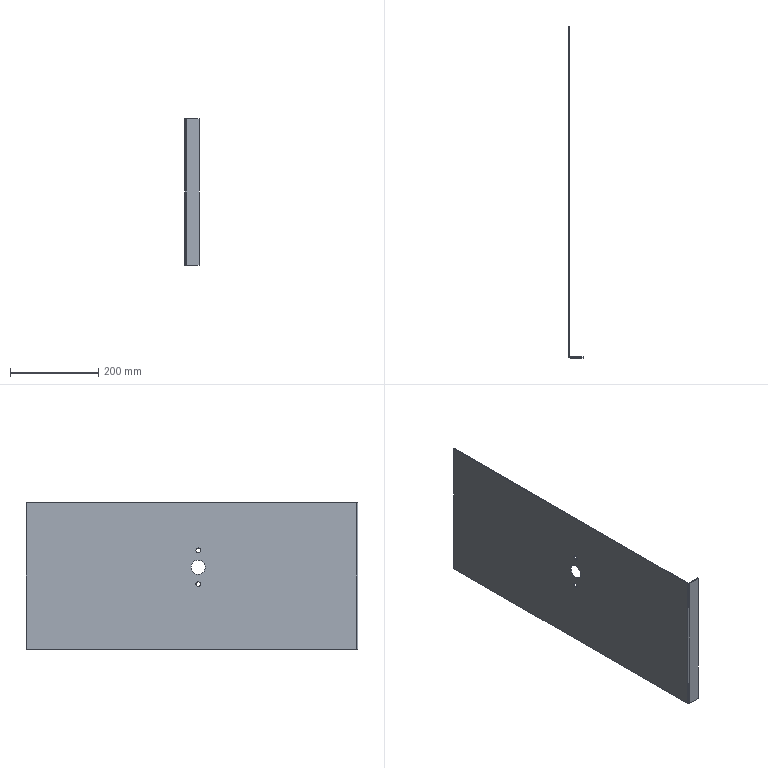Part | SolidWorks | features FlatPattern 1, ICE 1, SMBaseFlange 1, SheetMetal 1 | 1 solid | 20 faces | box 32 x 752 x 333 mm | volume 518361 mm3 | plane 12 | cylinder 8 | commonest cylinder face diameters 10.5 x4 32 x2 1.473 x1 5.473 x1
STEP:
#1=CARTESIAN_POINT('',(0.,87.126,63.5));
#2=VERTEX_POINT('',#1);
#3=CARTESIAN_POINT('',(0.,87.126,53.));
#4=VERTEX_POINT('',#3);
#5=CARTESIAN_POINT('',(0.,87.126,58.25));
#6=DIRECTION('',(1.,0.,0.));
#7=DIRECTION('',(0.,0.,-1.));
#8=AXIS2_PLACEMENT_3D('',#5,#6,#7);
#9=CIRCLE('',#8,5.25);
#10=EDGE_CURVE('',#2,#4,#9,.T.);
#11=ORIENTED_EDGE('',*,*,#10,.T.);
#12=CARTESIAN_POINT('',(-2.,87.126,53.));
#13=VERTEX_POINT('',#12);
#14=CARTESIAN_POINT('',(8.,87.126,53.));
#15=DIRECTION('',(-1.,0.,0.));
#16=VECTOR('',#15,1000.);
#17=LINE('',#14,#16);
#18=EDGE_CURVE('',#4,#13,#17,.T.);
#19=ORIENTED_EDGE('',*,*,#18,.T.);
#20=CARTESIAN_POINT('',(-2.,87.126,63.5));
#21=VERTEX_POINT('',#20);
#22=CARTESIAN_POINT('',(-2.,87.126,58.25));
#23=DIRECTION('',(-1.,0.,0.));
#24=DIRECTION('',(0.,0.,1.));
#25=AXIS2_PLACEMENT_3D('',#22,#23,#24);
#26=CIRCLE('',#25,5.25);
#27=EDGE_CURVE('',#13,#21,#26,.T.);
#28=ORIENTED_EDGE('',*,*,#27,.T.);
#29=CARTESIAN_POINT('',(8.,87.126,63.5));
#30=DIRECTION('',(-1.,0.,0.));
#31=VECTOR('',#30,1000.);
#32=LINE('',#29,#31);
#33=EDGE_CURVE('',#2,#21,#32,.T.);
#34=ORIENTED_EDGE('',*,*,#33,.F.);
#35=EDGE_LOOP('',(#11,#19,#28,#34));
#36=FACE_OUTER_BOUND('',#35,.T.);
#37=CARTESIAN_POINT('',(8.,87.126,58.25));
#38=DIRECTION('',(-1.,0.,0.));
#39=DIRECTION('',(0.,0.,1.));
#40=AXIS2_PLACEMENT_3D('',#37,#38,#39);
#41=CYLINDRICAL_SURFACE('',#40,5.25);
#42=ADVANCED_FACE('',(#36),#41,.F.);
#43=CARTESIAN_POINT('',(0.,87.126,-13.));
#44=VERTEX_POINT('',#43);
#45=CARTESIAN_POINT('',(0.,87.126,-23.5));
#46=VERTEX_POINT('',#45);
#47=CARTESIAN_POINT('',(0.,87.126,-18.25));
#48=DIRECTION('',(1.,0.,0.));
#49=DIRECTION('',(0.,0.,-1.));
#50=AXIS2_PLACEMENT_3D('',#47,#48,#49);
#51=CIRCLE('',#50,5.25);
#52=EDGE_CURVE('',#44,#46,#51,.T.);
#53=ORIENTED_EDGE('',*,*,#52,.T.);
#54=CARTESIAN_POINT('',(-2.,87.126,-23.5));
#55=VERTEX_POINT('',#54);
#56=CARTESIAN_POINT('',(8.,87.126,-23.5));
#57=DIRECTION('',(-1.,0.,0.));
#58=VECTOR('',#57,1000.);
#59=LINE('',#56,#58);
#60=EDGE_CURVE('',#46,#55,#59,.T.);
#61=ORIENTED_EDGE('',*,*,#60,.T.);
#62=CARTESIAN_POINT('',(-2.,87.126,-13.));
#63=VERTEX_POINT('',#62);
#64=CARTESIAN_POINT('',(-2.,87.126,-18.25));
#65=DIRECTION('',(-1.,0.,0.));
#66=DIRECTION('',(0.,0.,1.));
#67=AXIS2_PLACEMENT_3D('',#64,#65,#66);
#68=CIRCLE('',#67,5.25);
#69=EDGE_CURVE('',#55,#63,#68,.T.);
#70=ORIENTED_EDGE('',*,*,#69,.T.);
#71=CARTESIAN_POINT('',(8.,87.126,-13.));
#72=DIRECTION('',(-1.,0.,0.));
#73=VECTOR('',#72,1000.);
#74=LINE('',#71,#73);
#75=EDGE_CURVE('',#44,#63,#74,.T.);
#76=ORIENTED_EDGE('',*,*,#75,.F.);
#77=EDGE_LOOP('',(#53,#61,#70,#76));
#78=FACE_OUTER_BOUND('',#77,.T.);
#79=CARTESIAN_POINT('',(8.,87.126,-18.25));
#80=DIRECTION('',(-1.,0.,0.));
#81=DIRECTION('',(0.,0.,1.));
#82=AXIS2_PLACEMENT_3D('',#79,#80,#81);
#83=CYLINDRICAL_SURFACE('',#82,5.25);
#84=ADVANCED_FACE('',(#78),#83,.F.);
#85=CARTESIAN_POINT('',(0.,87.126,36.));
#86=VERTEX_POINT('',#85);
#87=CARTESIAN_POINT('',(0.,87.126,4.));
#88=VERTEX_POINT('',#87);
#89=CARTESIAN_POINT('',(0.,87.126,20.));
#90=DIRECTION('',(1.,0.,0.));
#91=DIRECTION('',(0.,0.,-1.));
#92=AXIS2_PLACEMENT_3D('',#89,#90,#91);
#93=CIRCLE('',#92,16.);
#94=EDGE_CURVE('',#86,#88,#93,.T.);
#95=ORIENTED_EDGE('',*,*,#94,.T.);
#96=CARTESIAN_POINT('',(-2.,87.126,4.));
#97=VERTEX_POINT('',#96);
#98=CARTESIAN_POINT('',(8.,87.126,4.));
#99=DIRECTION('',(-1.,0.,0.));
#100=VECTOR('',#99,1000.);
#101=LINE('',#98,#100);
#102=EDGE_CURVE('',#88,#97,#101,.T.);
#103=ORIENTED_EDGE('',*,*,#102,.T.);
#104=CARTESIAN_POINT('',(-2.,87.126,36.));
#105=VERTEX_POINT('',#104);
#106=CARTESIAN_POINT('',(-2.,87.126,20.));
#107=DIRECTION('',(-1.,0.,0.));
#108=DIRECTION('',(0.,0.,1.));
#109=AXIS2_PLACEMENT_3D('',#106,#107,#108);
#110=CIRCLE('',#109,16.);
#111=EDGE_CURVE('',#97,#105,#110,.T.);
#112=ORIENTED_EDGE('',*,*,#111,.T.);
#113=CARTESIAN_POINT('',(8.,87.126,36.));
#114=DIRECTION('',(-1.,0.,0.));
#115=VECTOR('',#114,1000.);
#116=LINE('',#113,#115);
#117=EDGE_CURVE('',#86,#105,#116,.T.);
#118=ORIENTED_EDGE('',*,*,#117,.F.);
#119=EDGE_LOOP('',(#95,#103,#112,#118));
#120=FACE_OUTER_BOUND('',#119,.T.);
#121=CARTESIAN_POINT('',(8.,87.126,20.));
#122=DIRECTION('',(-1.,0.,0.));
#123=DIRECTION('',(0.,0.,1.));
#124=AXIS2_PLACEMENT_3D('',#121,#122,#123);
#125=CYLINDRICAL_SURFACE('',#124,16.);
#126=ADVANCED_FACE('',(#120),#125,.F.);
#127=CARTESIAN_POINT('',(0.7366,-272.664,166.5));
#128=VERTEX_POINT('',#127);
#129=CARTESIAN_POINT('',(0.7366,-274.664,166.5));
#130=VERTEX_POINT('',#129);
#131=CARTESIAN_POINT('',(0.7366,-272.664,166.5));
#132=DIRECTION('',(0.,-1.,0.));
#133=VECTOR('',#132,1000.);
#134=LINE('',#131,#133);
#135=EDGE_CURVE('',#128,#130,#134,.T.);
#136=ORIENTED_EDGE('',*,*,#135,.F.);
#137=CARTESIAN_POINT('',(0.,-271.928,166.5));
#138=VERTEX_POINT('',#137);
#139=CARTESIAN_POINT('',(0.7366,-271.928,166.5));
#140=DIRECTION('',(0.,0.,1.));
#141=DIRECTION('',(-1.,0.,0.));
#142=AXIS2_PLACEMENT_3D('',#139,#140,#141);
#143=CIRCLE('',#142,0.7366);
#144=EDGE_CURVE('',#138,#128,#143,.T.);
#145=ORIENTED_EDGE('',*,*,#144,.F.);
#146=CARTESIAN_POINT('',(-2.,-271.928,166.5));
#147=VERTEX_POINT('',#146);
#148=CARTESIAN_POINT('',(-2.,-271.928,166.5));
#149=DIRECTION('',(1.,0.,0.));
#150=VECTOR('',#149,1000.);
#151=LINE('',#148,#150);
#152=EDGE_CURVE('',#147,#138,#151,.T.);
#153=ORIENTED_EDGE('',*,*,#152,.F.);
#154=CARTESIAN_POINT('',(0.7366,-271.928,166.5));
#155=DIRECTION('',(0.,0.,1.));
#156=DIRECTION('',(1.,0.,0.));
#157=AXIS2_PLACEMENT_3D('',#154,#155,#156);
#158=CIRCLE('',#157,2.737);
#159=EDGE_CURVE('',#147,#130,#158,.T.);
#160=ORIENTED_EDGE('',*,*,#159,.T.);
#161=EDGE_LOOP('',(#136,#145,#153,#160));
#162=FACE_OUTER_BOUND('',#161,.T.);
#163=CARTESIAN_POINT('',(0.7366,-272.664,166.5));
#164=DIRECTION('',(0.,0.,1.));
#165=DIRECTION('',(1.,0.,0.));
#166=AXIS2_PLACEMENT_3D('',#163,#164,#165);
#167=PLANE('',#166);
#168=ADVANCED_FACE('',(#162),#167,.T.);
#169=CARTESIAN_POINT('',(30.,-272.664,166.5));
#170=VERTEX_POINT('',#169);
#171=CARTESIAN_POINT('',(0.,-272.664,166.5));
#172=DIRECTION('',(1.,0.,0.));
#173=VECTOR('',#172,1000.);
#174=LINE('',#171,#173);
#175=EDGE_CURVE('',#128,#170,#174,.T.);
#176=ORIENTED_EDGE('',*,*,#175,.F.);
#177=ORIENTED_EDGE('',*,*,#135,.T.);
#178=CARTESIAN_POINT('',(30.,-274.664,166.5));
#179=VERTEX_POINT('',#178);
#180=CARTESIAN_POINT('',(0.,-274.664,166.5));
#181=DIRECTION('',(1.,0.,0.));
#182=VECTOR('',#181,1000.);
#183=LINE('',#180,#182);
#184=EDGE_CURVE('',#130,#179,#183,.T.);
#185=ORIENTED_EDGE('',*,*,#184,.T.);
#186=CARTESIAN_POINT('',(30.,-272.664,166.5));
#187=DIRECTION('',(0.,-1.,0.));
#188=VECTOR('',#187,1000.);
#189=LINE('',#186,#188);
#190=EDGE_CURVE('',#170,#179,#189,.T.);
#191=ORIENTED_EDGE('',*,*,#190,.F.);
#192=EDGE_LOOP('',(#176,#177,#185,#191));
#193=FACE_OUTER_BOUND('',#192,.T.);
#194=CARTESIAN_POINT('',(-2.,-271.928,166.5));
#195=DIRECTION('',(0.,0.,1.));
#196=DIRECTION('',(1.,0.,0.));
#197=AXIS2_PLACEMENT_3D('',#194,#195,#196);
#198=PLANE('',#197);
#199=ADVANCED_FACE('',(#193),#198,.T.);
#200=CARTESIAN_POINT('',(0.,-271.928,-166.5));
#201=VERTEX_POINT('',#200);
#202=CARTESIAN_POINT('',(-2.,-271.928,-166.5));
#203=VERTEX_POINT('',#202);
#204=CARTESIAN_POINT('',(0.,-271.928,-166.5));
#205=DIRECTION('',(-1.,0.,0.));
#206=VECTOR('',#205,1000.);
#207=LINE('',#204,#206);
#208=EDGE_CURVE('',#201,#203,#207,.T.);
#209=ORIENTED_EDGE('',*,*,#208,.F.);
#210=CARTESIAN_POINT('',(0.7366,-272.664,-166.5));
#211=VERTEX_POINT('',#210);
#212=CARTESIAN_POINT('',(0.7366,-271.928,-166.5));
#213=DIRECTION('',(0.,0.,1.));
#214=DIRECTION('',(-1.,0.,0.));
#215=AXIS2_PLACEMENT_3D('',#212,#213,#214);
#216=CIRCLE('',#215,0.7366);
#217=EDGE_CURVE('',#201,#211,#216,.T.);
#218=ORIENTED_EDGE('',*,*,#217,.T.);
#219=CARTESIAN_POINT('',(0.7366,-274.664,-166.5));
#220=VERTEX_POINT('',#219);
#221=CARTESIAN_POINT('',(0.7366,-274.664,-166.5));
#222=DIRECTION('',(0.,1.,0.));
#223=VECTOR('',#222,1000.);
#224=LINE('',#221,#223);
#225=EDGE_CURVE('',#220,#211,#224,.T.);
#226=ORIENTED_EDGE('',*,*,#225,.F.);
#227=CARTESIAN_POINT('',(0.7366,-271.928,-166.5));
#228=DIRECTION('',(0.,0.,1.));
#229=DIRECTION('',(1.,0.,0.));
#230=AXIS2_PLACEMENT_3D('',#227,#228,#229);
#231=CIRCLE('',#230,2.737);
#232=EDGE_CURVE('',#203,#220,#231,.T.);
#233=ORIENTED_EDGE('',*,*,#232,.F.);
#234=EDGE_LOOP('',(#209,#218,#226,#233));
#235=FACE_OUTER_BOUND('',#234,.T.);
#236=CARTESIAN_POINT('',(0.,-271.928,-166.5));
#237=DIRECTION('',(0.,0.,-1.));
#238=DIRECTION('',(-1.,0.,0.));
#239=AXIS2_PLACEMENT_3D('',#236,#237,#238);
#240=PLANE('',#239);
#241=ADVANCED_FACE('',(#235),#240,.T.);
#242=CARTESIAN_POINT('',(0.,477.336,-166.5));
#243=VERTEX_POINT('',#242);
#244=CARTESIAN_POINT('',(0.,477.336,-166.5));
#245=DIRECTION('',(0.,-1.,0.));
#246=VECTOR('',#245,1000.);
#247=LINE('',#244,#246);
#248=EDGE_CURVE('',#243,#201,#247,.T.);
#249=ORIENTED_EDGE('',*,*,#248,.T.);
#250=ORIENTED_EDGE('',*,*,#208,.T.);
#251=CARTESIAN_POINT('',(-2.,477.336,-166.5));
#252=VERTEX_POINT('',#251);
#253=CARTESIAN_POINT('',(-2.,477.336,-166.5));
#254=DIRECTION('',(0.,-1.,0.));
#255=VECTOR('',#254,1000.);
#256=LINE('',#253,#255);
#257=EDGE_CURVE('',#252,#203,#256,.T.);
#258=ORIENTED_EDGE('',*,*,#257,.F.);
#259=CARTESIAN_POINT('',(-2.,477.336,-166.5));
#260=DIRECTION('',(1.,0.,0.));
#261=VECTOR('',#260,1000.);
#262=LINE('',#259,#261);
#263=EDGE_CURVE('',#252,#243,#262,.T.);
#264=ORIENTED_EDGE('',*,*,#263,.T.);
#265=EDGE_LOOP('',(#249,#250,#258,#264));
#266=FACE_OUTER_BOUND('',#265,.T.);
#267=CARTESIAN_POINT('',(0.7366,-274.664,-166.5));
#268=DIRECTION('',(0.,0.,-1.));
#269=DIRECTION('',(-1.,0.,0.));
#270=AXIS2_PLACEMENT_3D('',#267,#268,#269);
#271=PLANE('',#270);
#272=ADVANCED_FACE('',(#266),#271,.T.);
#273=CARTESIAN_POINT('',(30.,-274.664,-166.5));
#274=VERTEX_POINT('',#273);
#275=CARTESIAN_POINT('',(0.,-274.664,-166.5));
#276=DIRECTION('',(1.,0.,0.));
#277=VECTOR('',#276,1000.);
#278=LINE('',#275,#277);
#279=EDGE_CURVE('',#220,#274,#278,.T.);
#280=ORIENTED_EDGE('',*,*,#279,.T.);
#281=CARTESIAN_POINT('',(30.,-274.664,166.5));
#282=DIRECTION('',(0.,0.,-1.));
#283=VECTOR('',#282,1000.);
#284=LINE('',#281,#283);
#285=EDGE_CURVE('',#179,#274,#284,.T.);
#286=ORIENTED_EDGE('',*,*,#285,.F.);
#287=ORIENTED_EDGE('',*,*,#184,.F.);
#288=CARTESIAN_POINT('',(0.7366,-274.664,166.5));
#289=DIRECTION('',(0.,0.,-1.));
#290=VECTOR('',#289,1000.);
#291=LINE('',#288,#290);
#292=EDGE_CURVE('',#130,#220,#291,.T.);
#293=ORIENTED_EDGE('',*,*,#292,.T.);
#294=EDGE_LOOP('',(#280,#286,#287,#293));
#295=FACE_OUTER_BOUND('',#294,.T.);
#296=CARTESIAN_POINT('',(0.,-274.664,166.5));
#297=DIRECTION('',(0.,1.,0.));
#298=DIRECTION('',(0.,0.,1.));
#299=AXIS2_PLACEMENT_3D('',#296,#297,#298);
#300=PLANE('',#299);
#301=ADVANCED_FACE('',(#295),#300,.F.);
#302=CARTESIAN_POINT('',(30.,-272.664,-166.5));
#303=VERTEX_POINT('',#302);
#304=CARTESIAN_POINT('',(30.,-272.664,-166.5));
#305=DIRECTION('',(0.,-1.,0.));
#306=VECTOR('',#305,1000.);
#307=LINE('',#304,#306);
#308=EDGE_CURVE('',#303,#274,#307,.T.);
#309=ORIENTED_EDGE('',*,*,#308,.F.);
#310=CARTESIAN_POINT('',(30.,-272.664,166.5));
#311=DIRECTION('',(0.,0.,-1.));
#312=VECTOR('',#311,1000.);
#313=LINE('',#310,#312);
#314=EDGE_CURVE('',#170,#303,#313,.T.);
#315=ORIENTED_EDGE('',*,*,#314,.F.);
#316=ORIENTED_EDGE('',*,*,#190,.T.);
#317=ORIENTED_EDGE('',*,*,#285,.T.);
#318=EDGE_LOOP('',(#309,#315,#316,#317));
#319=FACE_OUTER_BOUND('',#318,.T.);
#320=CARTESIAN_POINT('',(30.,-272.664,166.5));
#321=DIRECTION('',(1.,0.,0.));
#322=DIRECTION('',(0.,0.,-1.));
#323=AXIS2_PLACEMENT_3D('',#320,#321,#322);
#324=PLANE('',#323);
#325=ADVANCED_FACE('',(#319),#324,.T.);
#326=CARTESIAN_POINT('',(0.,-272.664,-166.5));
#327=DIRECTION('',(1.,0.,0.));
#328=VECTOR('',#327,1000.);
#329=LINE('',#326,#328);
#330=EDGE_CURVE('',#211,#303,#329,.T.);
#331=ORIENTED_EDGE('',*,*,#330,.F.);
#332=CARTESIAN_POINT('',(0.7366,-272.664,166.5));
#333=DIRECTION('',(0.,0.,-1.));
#334=VECTOR('',#333,1000.);
#335=LINE('',#332,#334);
#336=EDGE_CURVE('',#128,#211,#335,.T.);
#337=ORIENTED_EDGE('',*,*,#336,.F.);
#338=ORIENTED_EDGE('',*,*,#175,.T.);
#339=ORIENTED_EDGE('',*,*,#314,.T.);
#340=EDGE_LOOP('',(#331,#337,#338,#339));
#341=FACE_OUTER_BOUND('',#340,.T.);
#342=CARTESIAN_POINT('',(0.,-272.664,166.5));
#343=DIRECTION('',(0.,1.,0.));
#344=DIRECTION('',(0.,0.,1.));
#345=AXIS2_PLACEMENT_3D('',#342,#343,#344);
#346=PLANE('',#345);
#347=ADVANCED_FACE('',(#341),#346,.T.);
#348=ORIENTED_EDGE('',*,*,#217,.F.);
#349=CARTESIAN_POINT('',(0.,-271.928,166.5));
#350=DIRECTION('',(0.,0.,-1.));
#351=VECTOR('',#350,1000.);
#352=LINE('',#349,#351);
#353=EDGE_CURVE('',#138,#201,#352,.T.);
#354=ORIENTED_EDGE('',*,*,#353,.F.);
#355=ORIENTED_EDGE('',*,*,#144,.T.);
#356=ORIENTED_EDGE('',*,*,#336,.T.);
#357=EDGE_LOOP('',(#348,#354,#355,#356));
#358=FACE_OUTER_BOUND('',#357,.T.);
#359=CARTESIAN_POINT('',(0.7366,-271.928,166.5));
#360=DIRECTION('',(0.,0.,-1.));
#361=DIRECTION('',(-1.,0.,0.));
#362=AXIS2_PLACEMENT_3D('',#359,#360,#361);
#363=CYLINDRICAL_SURFACE('',#362,0.7366);
#364=ADVANCED_FACE('',(#358),#363,.F.);
#365=ORIENTED_EDGE('',*,*,#10,.F.);
#366=CARTESIAN_POINT('',(0.,87.126,58.25));
#367=DIRECTION('',(1.,0.,0.));
#368=DIRECTION('',(0.,0.,-1.));
#369=AXIS2_PLACEMENT_3D('',#366,#367,#368);
#370=CIRCLE('',#369,5.25);
#371=EDGE_CURVE('',#4,#2,#370,.T.);
#372=ORIENTED_EDGE('',*,*,#371,.F.);
#373=EDGE_LOOP('',(#365,#372));
#374=FACE_BOUND('',#373,.T.);
#375=ORIENTED_EDGE('',*,*,#52,.F.);
#376=CARTESIAN_POINT('',(0.,87.126,-18.25));
#377=DIRECTION('',(1.,0.,0.));
#378=DIRECTION('',(0.,0.,-1.));
#379=AXIS2_PLACEMENT_3D('',#376,#377,#378);
#380=CIRCLE('',#379,5.25);
#381=EDGE_CURVE('',#46,#44,#380,.T.);
#382=ORIENTED_EDGE('',*,*,#381,.F.);
#383=EDGE_LOOP('',(#375,#382));
#384=FACE_BOUND('',#383,.T.);
#385=ORIENTED_EDGE('',*,*,#94,.F.);
#386=CARTESIAN_POINT('',(0.,87.126,20.));
#387=DIRECTION('',(1.,0.,0.));
#388=DIRECTION('',(0.,0.,-1.));
#389=AXIS2_PLACEMENT_3D('',#386,#387,#388);
#390=CIRCLE('',#389,16.);
#391=EDGE_CURVE('',#88,#86,#390,.T.);
#392=ORIENTED_EDGE('',*,*,#391,.F.);
#393=EDGE_LOOP('',(#385,#392));
#394=FACE_BOUND('',#393,.T.);
#395=ORIENTED_EDGE('',*,*,#248,.F.);
#396=CARTESIAN_POINT('',(0.,477.336,166.5));
#397=VERTEX_POINT('',#396);
#398=CARTESIAN_POINT('',(0.,477.336,166.5));
#399=DIRECTION('',(0.,0.,-1.));
#400=VECTOR('',#399,1000.);
#401=LINE('',#398,#400);
#402=EDGE_CURVE('',#397,#243,#401,.T.);
#403=ORIENTED_EDGE('',*,*,#402,.F.);
#404=CARTESIAN_POINT('',(0.,477.336,166.5));
#405=DIRECTION('',(0.,-1.,0.));
#406=VECTOR('',#405,1000.);
#407=LINE('',#404,#406);
#408=EDGE_CURVE('',#397,#138,#407,.T.);
#409=ORIENTED_EDGE('',*,*,#408,.T.);
#410=ORIENTED_EDGE('',*,*,#353,.T.);
#411=EDGE_LOOP('',(#395,#403,#409,#410));
#412=FACE_OUTER_BOUND('',#411,.T.);
#413=CARTESIAN_POINT('',(0.,477.336,166.5));
#414=DIRECTION('',(1.,0.,0.));
#415=DIRECTION('',(0.,0.,-1.));
#416=AXIS2_PLACEMENT_3D('',#413,#414,#415);
#417=PLANE('',#416);
#418=ADVANCED_FACE('',(#374,#384,#394,#412),#417,.T.);
#419=ORIENTED_EDGE('',*,*,#263,.F.);
#420=CARTESIAN_POINT('',(-2.,477.336,166.5));
#421=VERTEX_POINT('',#420);
#422=CARTESIAN_POINT('',(-2.,477.336,166.5));
#423=DIRECTION('',(0.,0.,-1.));
#424=VECTOR('',#423,1000.);
#425=LINE('',#422,#424);
#426=EDGE_CURVE('',#421,#252,#425,.T.);
#427=ORIENTED_EDGE('',*,*,#426,.F.);
#428=CARTESIAN_POINT('',(-2.,477.336,166.5));
#429=DIRECTION('',(1.,0.,0.));
#430=VECTOR('',#429,1000.);
#431=LINE('',#428,#430);
#432=EDGE_CURVE('',#421,#397,#431,.T.);
#433=ORIENTED_EDGE('',*,*,#432,.T.);
#434=ORIENTED_EDGE('',*,*,#402,.T.);
#435=EDGE_LOOP('',(#419,#427,#433,#434));
#436=FACE_OUTER_BOUND('',#435,.T.);
#437=CARTESIAN_POINT('',(-2.,477.336,166.5));
#438=DIRECTION('',(0.,1.,0.));
#439=DIRECTION('',(0.,0.,1.));
#440=AXIS2_PLACEMENT_3D('',#437,#438,#439);
#441=PLANE('',#440);
#442=ADVANCED_FACE('',(#436),#441,.T.);
#443=CARTESIAN_POINT('',(-2.,87.126,58.25));
#444=DIRECTION('',(-1.,0.,0.));
#445=DIRECTION('',(0.,0.,1.));
#446=AXIS2_PLACEMENT_3D('',#443,#444,#445);
#447=CIRCLE('',#446,5.25);
#448=EDGE_CURVE('',#21,#13,#447,.T.);
#449=ORIENTED_EDGE('',*,*,#448,.F.);
#450=ORIENTED_EDGE('',*,*,#27,.F.);
#451=EDGE_LOOP('',(#449,#450));
#452=FACE_BOUND('',#451,.T.);
#453=CARTESIAN_POINT('',(-2.,87.126,-18.25));
#454=DIRECTION('',(-1.,0.,0.));
#455=DIRECTION('',(0.,0.,1.));
#456=AXIS2_PLACEMENT_3D('',#453,#454,#455);
#457=CIRCLE('',#456,5.25);
#458=EDGE_CURVE('',#63,#55,#457,.T.);
#459=ORIENTED_EDGE('',*,*,#458,.F.);
#460=ORIENTED_EDGE('',*,*,#69,.F.);
#461=EDGE_LOOP('',(#459,#460));
#462=FACE_BOUND('',#461,.T.);
#463=CARTESIAN_POINT('',(-2.,87.126,20.));
#464=DIRECTION('',(-1.,0.,0.));
#465=DIRECTION('',(0.,0.,1.));
#466=AXIS2_PLACEMENT_3D('',#463,#464,#465);
#467=CIRCLE('',#466,16.);
#468=EDGE_CURVE('',#105,#97,#467,.T.);
#469=ORIENTED_EDGE('',*,*,#468,.F.);
#470=ORIENTED_EDGE('',*,*,#111,.F.);
#471=EDGE_LOOP('',(#469,#470));
#472=FACE_BOUND('',#471,.T.);
#473=ORIENTED_EDGE('',*,*,#257,.T.);
#474=CARTESIAN_POINT('',(-2.,-271.928,166.5));
#475=DIRECTION('',(0.,0.,-1.));
#476=VECTOR('',#475,1000.);
#477=LINE('',#474,#476);
#478=EDGE_CURVE('',#147,#203,#477,.T.);
#479=ORIENTED_EDGE('',*,*,#478,.F.);
#480=CARTESIAN_POINT('',(-2.,477.336,166.5));
#481=DIRECTION('',(0.,-1.,0.));
#482=VECTOR('',#481,1000.);
#483=LINE('',#480,#482);
#484=EDGE_CURVE('',#421,#147,#483,.T.);
#485=ORIENTED_EDGE('',*,*,#484,.F.);
#486=ORIENTED_EDGE('',*,*,#426,.T.);
#487=EDGE_LOOP('',(#473,#479,#485,#486));
#488=FACE_OUTER_BOUND('',#487,.T.);
#489=CARTESIAN_POINT('',(-2.,477.336,166.5));
#490=DIRECTION('',(1.,0.,0.));
#491=DIRECTION('',(0.,0.,-1.));
#492=AXIS2_PLACEMENT_3D('',#489,#490,#491);
#493=PLANE('',#492);
#494=ADVANCED_FACE('',(#452,#462,#472,#488),#493,.F.);
#495=ORIENTED_EDGE('',*,*,#232,.T.);
#496=ORIENTED_EDGE('',*,*,#292,.F.);
#497=ORIENTED_EDGE('',*,*,#159,.F.);
#498=ORIENTED_EDGE('',*,*,#478,.T.);
#499=EDGE_LOOP('',(#495,#496,#497,#498));
#500=FACE_OUTER_BOUND('',#499,.T.);
#501=CARTESIAN_POINT('',(0.7366,-271.928,166.5));
#502=DIRECTION('',(0.,0.,-1.));
#503=DIRECTION('',(-1.,0.,0.));
#504=AXIS2_PLACEMENT_3D('',#501,#502,#503);
#505=CYLINDRICAL_SURFACE('',#504,2.737);
#506=ADVANCED_FACE('',(#500),#505,.T.);
#507=ORIENTED_EDGE('',*,*,#484,.T.);
#508=ORIENTED_EDGE('',*,*,#152,.T.);
#509=ORIENTED_EDGE('',*,*,#408,.F.);
#510=ORIENTED_EDGE('',*,*,#432,.F.);
#511=EDGE_LOOP('',(#507,#508,#509,#510));
#512=FACE_OUTER_BOUND('',#511,.T.);
#513=CARTESIAN_POINT('',(0.7366,-271.928,166.5));
#514=DIRECTION('',(0.,0.,-1.));
#515=DIRECTION('',(-1.,0.,0.));
#516=AXIS2_PLACEMENT_3D('',#513,#514,#515);
#517=PLANE('',#516);
#518=ADVANCED_FACE('',(#512),#517,.F.);
#519=ORIENTED_EDGE('',*,*,#279,.F.);
#520=ORIENTED_EDGE('',*,*,#225,.T.);
#521=ORIENTED_EDGE('',*,*,#330,.T.);
#522=ORIENTED_EDGE('',*,*,#308,.T.);
#523=EDGE_LOOP('',(#519,#520,#521,#522));
#524=FACE_OUTER_BOUND('',#523,.T.);
#525=CARTESIAN_POINT('',(0.7366,-271.928,-166.5));
#526=DIRECTION('',(0.,0.,-1.));
#527=DIRECTION('',(-1.,0.,0.));
#528=AXIS2_PLACEMENT_3D('',#525,#526,#527);
#529=PLANE('',#528);
#530=ADVANCED_FACE('',(#524),#529,.T.);
#531=ORIENTED_EDGE('',*,*,#102,.F.);
#532=ORIENTED_EDGE('',*,*,#391,.T.);
#533=ORIENTED_EDGE('',*,*,#117,.T.);
#534=ORIENTED_EDGE('',*,*,#468,.T.);
#535=EDGE_LOOP('',(#531,#532,#533,#534));
#536=FACE_OUTER_BOUND('',#535,.T.);
#537=CARTESIAN_POINT('',(8.,87.126,20.));
#538=DIRECTION('',(-1.,0.,0.));
#539=DIRECTION('',(0.,0.,1.));
#540=AXIS2_PLACEMENT_3D('',#537,#538,#539);
#541=CYLINDRICAL_SURFACE('',#540,16.);
#542=ADVANCED_FACE('',(#536),#541,.F.);
#543=ORIENTED_EDGE('',*,*,#60,.F.);
#544=ORIENTED_EDGE('',*,*,#381,.T.);
#545=ORIENTED_EDGE('',*,*,#75,.T.);
#546=ORIENTED_EDGE('',*,*,#458,.T.);
#547=EDGE_LOOP('',(#543,#544,#545,#546));
#548=FACE_OUTER_BOUND('',#547,.T.);
#549=CARTESIAN_POINT('',(8.,87.126,-18.25));
#550=DIRECTION('',(-1.,0.,0.));
#551=DIRECTION('',(0.,0.,1.));
#552=AXIS2_PLACEMENT_3D('',#549,#550,#551);
#553=CYLINDRICAL_SURFACE('',#552,5.25);
#554=ADVANCED_FACE('',(#548),#553,.F.);
#555=ORIENTED_EDGE('',*,*,#18,.F.);
#556=ORIENTED_EDGE('',*,*,#371,.T.);
#557=ORIENTED_EDGE('',*,*,#33,.T.);
#558=ORIENTED_EDGE('',*,*,#448,.T.);
#559=EDGE_LOOP('',(#555,#556,#557,#558));
#560=FACE_OUTER_BOUND('',#559,.T.);
#561=CARTESIAN_POINT('',(8.,87.126,58.25));
#562=DIRECTION('',(-1.,0.,0.));
#563=DIRECTION('',(0.,0.,1.));
#564=AXIS2_PLACEMENT_3D('',#561,#562,#563);
#565=CYLINDRICAL_SURFACE('',#564,5.25);
#566=ADVANCED_FACE('',(#560),#565,.F.);
#567=CLOSED_SHELL('',(#42,#84,#126,#168,#199,#241,#272,#301,#325,#347,#364,#418,#442,#494,#506,#518,#530,#542,#554,#566));
#568=MANIFOLD_SOLID_BREP('',#567);
#569=CARTESIAN_POINT('',(0.,0.,0.));
#570=DIRECTION('',(0.,0.,1.));
#571=DIRECTION('',(1.,0.,0.));
#572=AXIS2_PLACEMENT_3D('',#569,#570,#571);
#573=(LENGTH_UNIT()NAMED_UNIT(*)SI_UNIT(.MILLI.,.METRE.));
#574=UNCERTAINTY_MEASURE_WITH_UNIT(LENGTH_MEASURE(0.00001),#573,'','');
#575=(NAMED_UNIT(*)PLANE_ANGLE_UNIT()SI_UNIT($,.RADIAN.));
#576=(NAMED_UNIT(*)SI_UNIT($,.STERADIAN.)SOLID_ANGLE_UNIT());
#577=(GEOMETRIC_REPRESENTATION_CONTEXT(3)GLOBAL_UNCERTAINTY_ASSIGNED_CONTEXT((#574))GLOBAL_UNIT_ASSIGNED_CONTEXT((#573,#575,#576))REPRESENTATION_CONTEXT('',''));
#578=ADVANCED_BREP_SHAPE_REPRESENTATION('',(#568,#572),#577);